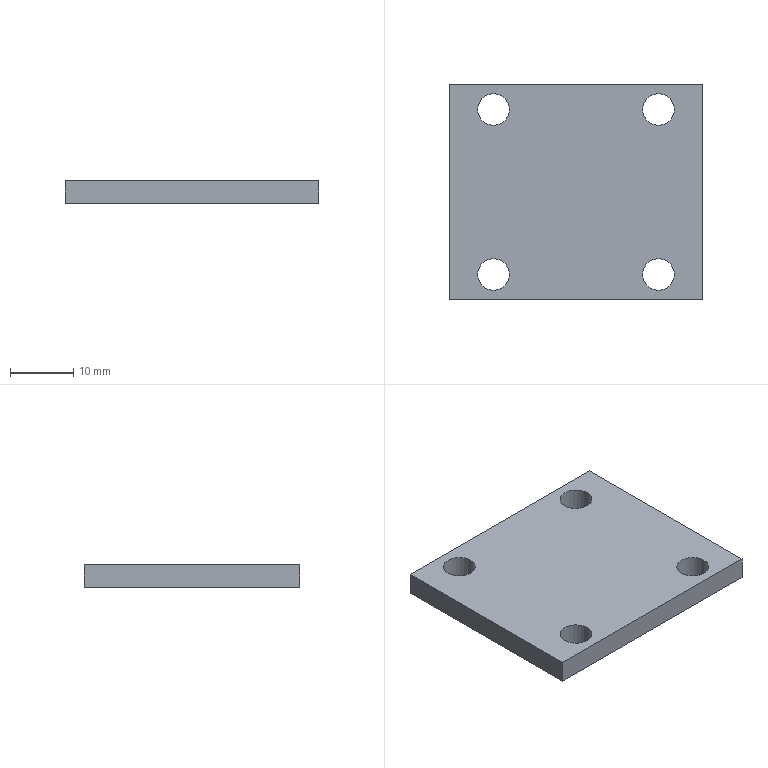Part | NX | 1 solid | 14 faces | box 40 x 34 x 3.6 mm | volume 4613 mm3 | cylinder 8 | plane 6 | commonest cylinder face diameters 5 x8
STEP:
#1=CARTESIAN_POINT('',(0.,0.,-5.));
#2=VERTEX_POINT('',#1);
#3=CARTESIAN_POINT('',(0.,-34.,-5.));
#4=VERTEX_POINT('',#3);
#5=CARTESIAN_POINT('',(0.,0.,-5.));
#6=DIRECTION('',(0.,-1.,0.));
#7=VECTOR('',#6,1000.);
#8=LINE('',#5,#7);
#9=EDGE_CURVE('',#2,#4,#8,.T.);
#10=ORIENTED_EDGE('',*,*,#9,.T.);
#11=CARTESIAN_POINT('',(40.,-34.,-5.));
#12=VERTEX_POINT('',#11);
#13=CARTESIAN_POINT('',(0.,-34.,-5.));
#14=DIRECTION('',(1.,0.,0.));
#15=VECTOR('',#14,1000.);
#16=LINE('',#13,#15);
#17=EDGE_CURVE('',#4,#12,#16,.T.);
#18=ORIENTED_EDGE('',*,*,#17,.T.);
#19=CARTESIAN_POINT('',(40.,0.,-5.));
#20=VERTEX_POINT('',#19);
#21=CARTESIAN_POINT('',(40.,0.,-5.));
#22=DIRECTION('',(0.,1.,0.));
#23=VECTOR('',#22,1000.);
#24=LINE('',#21,#23);
#25=EDGE_CURVE('',#12,#20,#24,.T.);
#26=ORIENTED_EDGE('',*,*,#25,.T.);
#27=CARTESIAN_POINT('',(0.,0.,-5.));
#28=DIRECTION('',(-1.,0.,0.));
#29=VECTOR('',#28,1000.);
#30=LINE('',#27,#29);
#31=EDGE_CURVE('',#20,#2,#30,.T.);
#32=ORIENTED_EDGE('',*,*,#31,.T.);
#33=EDGE_LOOP('',(#10,#18,#26,#32));
#34=FACE_BOUND('',#33,.T.);
#35=CARTESIAN_POINT('',(4.5,-4.,-5.));
#36=VERTEX_POINT('',#35);
#37=CARTESIAN_POINT('',(9.5,-4.,-5.));
#38=VERTEX_POINT('',#37);
#39=CARTESIAN_POINT('',(7.,-4.,-5.));
#40=DIRECTION('',(0.,0.,-1.));
#41=DIRECTION('',(-1.,0.,0.));
#42=AXIS2_PLACEMENT_3D('',#39,#40,#41);
#43=CIRCLE('',#42,2.5);
#44=EDGE_CURVE('',#36,#38,#43,.T.);
#45=ORIENTED_EDGE('',*,*,#44,.T.);
#46=CARTESIAN_POINT('',(7.,-4.,-5.));
#47=DIRECTION('',(0.,0.,-1.));
#48=DIRECTION('',(-1.,0.,0.));
#49=AXIS2_PLACEMENT_3D('',#46,#47,#48);
#50=CIRCLE('',#49,2.5);
#51=EDGE_CURVE('',#38,#36,#50,.T.);
#52=ORIENTED_EDGE('',*,*,#51,.T.);
#53=EDGE_LOOP('',(#45,#52));
#54=FACE_BOUND('',#53,.T.);
#55=CARTESIAN_POINT('',(4.5,-30.,-5.));
#56=VERTEX_POINT('',#55);
#57=CARTESIAN_POINT('',(9.5,-30.,-5.));
#58=VERTEX_POINT('',#57);
#59=CARTESIAN_POINT('',(7.,-30.,-5.));
#60=DIRECTION('',(0.,0.,-1.));
#61=DIRECTION('',(-1.,0.,0.));
#62=AXIS2_PLACEMENT_3D('',#59,#60,#61);
#63=CIRCLE('',#62,2.5);
#64=EDGE_CURVE('',#56,#58,#63,.T.);
#65=ORIENTED_EDGE('',*,*,#64,.T.);
#66=CARTESIAN_POINT('',(7.,-30.,-5.));
#67=DIRECTION('',(0.,0.,-1.));
#68=DIRECTION('',(-1.,0.,0.));
#69=AXIS2_PLACEMENT_3D('',#66,#67,#68);
#70=CIRCLE('',#69,2.5);
#71=EDGE_CURVE('',#58,#56,#70,.T.);
#72=ORIENTED_EDGE('',*,*,#71,.T.);
#73=EDGE_LOOP('',(#65,#72));
#74=FACE_BOUND('',#73,.T.);
#75=CARTESIAN_POINT('',(35.5,-4.,-5.));
#76=VERTEX_POINT('',#75);
#77=CARTESIAN_POINT('',(30.5,-4.,-5.));
#78=VERTEX_POINT('',#77);
#79=CARTESIAN_POINT('',(33.,-4.,-5.));
#80=DIRECTION('',(0.,0.,-1.));
#81=DIRECTION('',(-1.,0.,0.));
#82=AXIS2_PLACEMENT_3D('',#79,#80,#81);
#83=CIRCLE('',#82,2.5);
#84=EDGE_CURVE('',#76,#78,#83,.T.);
#85=ORIENTED_EDGE('',*,*,#84,.T.);
#86=CARTESIAN_POINT('',(33.,-4.,-5.));
#87=DIRECTION('',(0.,0.,-1.));
#88=DIRECTION('',(-1.,0.,0.));
#89=AXIS2_PLACEMENT_3D('',#86,#87,#88);
#90=CIRCLE('',#89,2.5);
#91=EDGE_CURVE('',#78,#76,#90,.T.);
#92=ORIENTED_EDGE('',*,*,#91,.T.);
#93=EDGE_LOOP('',(#85,#92));
#94=FACE_BOUND('',#93,.T.);
#95=CARTESIAN_POINT('',(30.5,-30.,-5.));
#96=VERTEX_POINT('',#95);
#97=CARTESIAN_POINT('',(35.5,-30.,-5.));
#98=VERTEX_POINT('',#97);
#99=CARTESIAN_POINT('',(33.,-30.,-5.));
#100=DIRECTION('',(0.,0.,-1.));
#101=DIRECTION('',(-1.,0.,0.));
#102=AXIS2_PLACEMENT_3D('',#99,#100,#101);
#103=CIRCLE('',#102,2.5);
#104=EDGE_CURVE('',#96,#98,#103,.T.);
#105=ORIENTED_EDGE('',*,*,#104,.T.);
#106=CARTESIAN_POINT('',(33.,-30.,-5.));
#107=DIRECTION('',(0.,0.,-1.));
#108=DIRECTION('',(-1.,0.,0.));
#109=AXIS2_PLACEMENT_3D('',#106,#107,#108);
#110=CIRCLE('',#109,2.5);
#111=EDGE_CURVE('',#98,#96,#110,.T.);
#112=ORIENTED_EDGE('',*,*,#111,.T.);
#113=EDGE_LOOP('',(#105,#112));
#114=FACE_BOUND('',#113,.T.);
#115=CARTESIAN_POINT('',(0.,0.,-5.));
#116=DIRECTION('',(0.,0.,1.));
#117=DIRECTION('',(1.,0.,0.));
#118=AXIS2_PLACEMENT_3D('',#115,#116,#117);
#119=PLANE('',#118);
#120=ADVANCED_FACE('',(#34,#54,#74,#94,#114),#119,.T.);
#121=CARTESIAN_POINT('',(0.,0.,-8.6));
#122=VERTEX_POINT('',#121);
#123=CARTESIAN_POINT('',(0.,-34.,-8.6));
#124=VERTEX_POINT('',#123);
#125=CARTESIAN_POINT('',(0.,0.,-8.6));
#126=DIRECTION('',(0.,-1.,0.));
#127=VECTOR('',#126,1000.);
#128=LINE('',#125,#127);
#129=EDGE_CURVE('',#122,#124,#128,.T.);
#130=ORIENTED_EDGE('',*,*,#129,.T.);
#131=CARTESIAN_POINT('',(0.,-34.,0.));
#132=DIRECTION('',(0.,0.,-1.));
#133=VECTOR('',#132,1000.);
#134=LINE('',#131,#133);
#135=EDGE_CURVE('',#4,#124,#134,.T.);
#136=ORIENTED_EDGE('',*,*,#135,.F.);
#137=ORIENTED_EDGE('',*,*,#9,.F.);
#138=CARTESIAN_POINT('',(0.,0.,0.));
#139=DIRECTION('',(0.,0.,1.));
#140=VECTOR('',#139,1000.);
#141=LINE('',#138,#140);
#142=EDGE_CURVE('',#122,#2,#141,.T.);
#143=ORIENTED_EDGE('',*,*,#142,.F.);
#144=EDGE_LOOP('',(#130,#136,#137,#143));
#145=FACE_BOUND('',#144,.T.);
#146=CARTESIAN_POINT('',(0.,0.,0.));
#147=DIRECTION('',(-1.,0.,0.));
#148=DIRECTION('',(0.,0.,1.));
#149=AXIS2_PLACEMENT_3D('',#146,#147,#148);
#150=PLANE('',#149);
#151=ADVANCED_FACE('',(#145),#150,.T.);
#152=CARTESIAN_POINT('',(40.,0.,-8.6));
#153=VERTEX_POINT('',#152);
#154=CARTESIAN_POINT('',(0.,0.,-8.6));
#155=DIRECTION('',(-1.,0.,0.));
#156=VECTOR('',#155,1000.);
#157=LINE('',#154,#156);
#158=EDGE_CURVE('',#153,#122,#157,.T.);
#159=ORIENTED_EDGE('',*,*,#158,.T.);
#160=ORIENTED_EDGE('',*,*,#142,.T.);
#161=ORIENTED_EDGE('',*,*,#31,.F.);
#162=CARTESIAN_POINT('',(40.,0.,0.));
#163=DIRECTION('',(0.,0.,-1.));
#164=VECTOR('',#163,1000.);
#165=LINE('',#162,#164);
#166=EDGE_CURVE('',#20,#153,#165,.T.);
#167=ORIENTED_EDGE('',*,*,#166,.T.);
#168=EDGE_LOOP('',(#159,#160,#161,#167));
#169=FACE_BOUND('',#168,.T.);
#170=CARTESIAN_POINT('',(40.,0.,0.));
#171=DIRECTION('',(0.,1.,0.));
#172=DIRECTION('',(1.,0.,0.));
#173=AXIS2_PLACEMENT_3D('',#170,#171,#172);
#174=PLANE('',#173);
#175=ADVANCED_FACE('',(#169),#174,.T.);
#176=CARTESIAN_POINT('',(40.,-34.,-8.6));
#177=VERTEX_POINT('',#176);
#178=CARTESIAN_POINT('',(40.,0.,-8.6));
#179=DIRECTION('',(0.,1.,0.));
#180=VECTOR('',#179,1000.);
#181=LINE('',#178,#180);
#182=EDGE_CURVE('',#177,#153,#181,.T.);
#183=ORIENTED_EDGE('',*,*,#182,.T.);
#184=ORIENTED_EDGE('',*,*,#166,.F.);
#185=ORIENTED_EDGE('',*,*,#25,.F.);
#186=CARTESIAN_POINT('',(40.,-34.,0.));
#187=DIRECTION('',(0.,0.,1.));
#188=VECTOR('',#187,1000.);
#189=LINE('',#186,#188);
#190=EDGE_CURVE('',#177,#12,#189,.T.);
#191=ORIENTED_EDGE('',*,*,#190,.F.);
#192=EDGE_LOOP('',(#183,#184,#185,#191));
#193=FACE_BOUND('',#192,.T.);
#194=CARTESIAN_POINT('',(40.,-34.,0.));
#195=DIRECTION('',(1.,0.,0.));
#196=DIRECTION('',(0.,1.,0.));
#197=AXIS2_PLACEMENT_3D('',#194,#195,#196);
#198=PLANE('',#197);
#199=ADVANCED_FACE('',(#193),#198,.T.);
#200=CARTESIAN_POINT('',(0.,-34.,-8.6));
#201=DIRECTION('',(1.,0.,0.));
#202=VECTOR('',#201,1000.);
#203=LINE('',#200,#202);
#204=EDGE_CURVE('',#124,#177,#203,.T.);
#205=ORIENTED_EDGE('',*,*,#204,.T.);
#206=ORIENTED_EDGE('',*,*,#190,.T.);
#207=ORIENTED_EDGE('',*,*,#17,.F.);
#208=ORIENTED_EDGE('',*,*,#135,.T.);
#209=EDGE_LOOP('',(#205,#206,#207,#208));
#210=FACE_BOUND('',#209,.T.);
#211=CARTESIAN_POINT('',(0.,-34.,0.));
#212=DIRECTION('',(0.,-1.,0.));
#213=DIRECTION('',(0.,0.,-1.));
#214=AXIS2_PLACEMENT_3D('',#211,#212,#213);
#215=PLANE('',#214);
#216=ADVANCED_FACE('',(#210),#215,.T.);
#217=ORIENTED_EDGE('',*,*,#129,.F.);
#218=ORIENTED_EDGE('',*,*,#158,.F.);
#219=ORIENTED_EDGE('',*,*,#182,.F.);
#220=ORIENTED_EDGE('',*,*,#204,.F.);
#221=EDGE_LOOP('',(#217,#218,#219,#220));
#222=FACE_BOUND('',#221,.T.);
#223=CARTESIAN_POINT('',(9.5,-4.,-8.6));
#224=VERTEX_POINT('',#223);
#225=CARTESIAN_POINT('',(4.5,-4.,-8.6));
#226=VERTEX_POINT('',#225);
#227=CARTESIAN_POINT('',(7.,-4.,-8.6));
#228=DIRECTION('',(0.,0.,-1.));
#229=DIRECTION('',(-1.,0.,0.));
#230=AXIS2_PLACEMENT_3D('',#227,#228,#229);
#231=CIRCLE('',#230,2.5);
#232=EDGE_CURVE('',#224,#226,#231,.T.);
#233=ORIENTED_EDGE('',*,*,#232,.F.);
#234=CARTESIAN_POINT('',(7.,-4.,-8.6));
#235=DIRECTION('',(0.,0.,-1.));
#236=DIRECTION('',(-1.,0.,0.));
#237=AXIS2_PLACEMENT_3D('',#234,#235,#236);
#238=CIRCLE('',#237,2.5);
#239=EDGE_CURVE('',#226,#224,#238,.T.);
#240=ORIENTED_EDGE('',*,*,#239,.F.);
#241=EDGE_LOOP('',(#233,#240));
#242=FACE_BOUND('',#241,.T.);
#243=CARTESIAN_POINT('',(4.5,-30.,-8.6));
#244=VERTEX_POINT('',#243);
#245=CARTESIAN_POINT('',(9.5,-30.,-8.6));
#246=VERTEX_POINT('',#245);
#247=CARTESIAN_POINT('',(7.,-30.,-8.6));
#248=DIRECTION('',(0.,0.,-1.));
#249=DIRECTION('',(-1.,0.,0.));
#250=AXIS2_PLACEMENT_3D('',#247,#248,#249);
#251=CIRCLE('',#250,2.5);
#252=EDGE_CURVE('',#244,#246,#251,.T.);
#253=ORIENTED_EDGE('',*,*,#252,.F.);
#254=CARTESIAN_POINT('',(7.,-30.,-8.6));
#255=DIRECTION('',(0.,0.,-1.));
#256=DIRECTION('',(-1.,0.,0.));
#257=AXIS2_PLACEMENT_3D('',#254,#255,#256);
#258=CIRCLE('',#257,2.5);
#259=EDGE_CURVE('',#246,#244,#258,.T.);
#260=ORIENTED_EDGE('',*,*,#259,.F.);
#261=EDGE_LOOP('',(#253,#260));
#262=FACE_BOUND('',#261,.T.);
#263=CARTESIAN_POINT('',(35.5,-4.,-8.6));
#264=VERTEX_POINT('',#263);
#265=CARTESIAN_POINT('',(30.5,-4.,-8.6));
#266=VERTEX_POINT('',#265);
#267=CARTESIAN_POINT('',(33.,-4.,-8.6));
#268=DIRECTION('',(0.,0.,-1.));
#269=DIRECTION('',(-1.,0.,0.));
#270=AXIS2_PLACEMENT_3D('',#267,#268,#269);
#271=CIRCLE('',#270,2.5);
#272=EDGE_CURVE('',#264,#266,#271,.T.);
#273=ORIENTED_EDGE('',*,*,#272,.F.);
#274=CARTESIAN_POINT('',(33.,-4.,-8.6));
#275=DIRECTION('',(0.,0.,-1.));
#276=DIRECTION('',(-1.,0.,0.));
#277=AXIS2_PLACEMENT_3D('',#274,#275,#276);
#278=CIRCLE('',#277,2.5);
#279=EDGE_CURVE('',#266,#264,#278,.T.);
#280=ORIENTED_EDGE('',*,*,#279,.F.);
#281=EDGE_LOOP('',(#273,#280));
#282=FACE_BOUND('',#281,.T.);
#283=CARTESIAN_POINT('',(35.5,-30.,-8.6));
#284=VERTEX_POINT('',#283);
#285=CARTESIAN_POINT('',(30.5,-30.,-8.6));
#286=VERTEX_POINT('',#285);
#287=CARTESIAN_POINT('',(33.,-30.,-8.6));
#288=DIRECTION('',(0.,0.,-1.));
#289=DIRECTION('',(-1.,0.,0.));
#290=AXIS2_PLACEMENT_3D('',#287,#288,#289);
#291=CIRCLE('',#290,2.5);
#292=EDGE_CURVE('',#284,#286,#291,.T.);
#293=ORIENTED_EDGE('',*,*,#292,.F.);
#294=CARTESIAN_POINT('',(33.,-30.,-8.6));
#295=DIRECTION('',(0.,0.,-1.));
#296=DIRECTION('',(-1.,0.,0.));
#297=AXIS2_PLACEMENT_3D('',#294,#295,#296);
#298=CIRCLE('',#297,2.5);
#299=EDGE_CURVE('',#286,#284,#298,.T.);
#300=ORIENTED_EDGE('',*,*,#299,.F.);
#301=EDGE_LOOP('',(#293,#300));
#302=FACE_BOUND('',#301,.T.);
#303=CARTESIAN_POINT('',(0.,0.,-8.6));
#304=DIRECTION('',(0.,0.,1.));
#305=DIRECTION('',(1.,0.,0.));
#306=AXIS2_PLACEMENT_3D('',#303,#304,#305);
#307=PLANE('',#306);
#308=ADVANCED_FACE('',(#222,#242,#262,#282,#302),#307,.F.);
#309=ORIENTED_EDGE('',*,*,#232,.T.);
#310=CARTESIAN_POINT('',(4.5,-4.,3.7));
#311=DIRECTION('',(0.,0.,-1.));
#312=VECTOR('',#311,1000.);
#313=LINE('',#310,#312);
#314=EDGE_CURVE('',#226,#36,#313,.F.);
#315=ORIENTED_EDGE('',*,*,#314,.T.);
#316=ORIENTED_EDGE('',*,*,#51,.F.);
#317=CARTESIAN_POINT('',(9.5,-4.,3.7));
#318=DIRECTION('',(0.,0.,-1.));
#319=VECTOR('',#318,1000.);
#320=LINE('',#317,#319);
#321=EDGE_CURVE('',#224,#38,#320,.F.);
#322=ORIENTED_EDGE('',*,*,#321,.F.);
#323=EDGE_LOOP('',(#309,#315,#316,#322));
#324=FACE_BOUND('',#323,.T.);
#325=CARTESIAN_POINT('',(7.,-4.,3.7));
#326=DIRECTION('',(0.,0.,-1.));
#327=DIRECTION('',(-1.,0.,0.));
#328=AXIS2_PLACEMENT_3D('',#325,#326,#327);
#329=CYLINDRICAL_SURFACE('',#328,2.5);
#330=ADVANCED_FACE('',(#324),#329,.F.);
#331=ORIENTED_EDGE('',*,*,#272,.T.);
#332=CARTESIAN_POINT('',(30.5,-4.,3.7));
#333=DIRECTION('',(0.,0.,-1.));
#334=VECTOR('',#333,1000.);
#335=LINE('',#332,#334);
#336=EDGE_CURVE('',#266,#78,#335,.F.);
#337=ORIENTED_EDGE('',*,*,#336,.T.);
#338=ORIENTED_EDGE('',*,*,#84,.F.);
#339=CARTESIAN_POINT('',(35.5,-4.,3.7));
#340=DIRECTION('',(0.,0.,-1.));
#341=VECTOR('',#340,1000.);
#342=LINE('',#339,#341);
#343=EDGE_CURVE('',#264,#76,#342,.F.);
#344=ORIENTED_EDGE('',*,*,#343,.F.);
#345=EDGE_LOOP('',(#331,#337,#338,#344));
#346=FACE_BOUND('',#345,.T.);
#347=CARTESIAN_POINT('',(33.,-4.,3.7));
#348=DIRECTION('',(0.,0.,-1.));
#349=DIRECTION('',(-1.,0.,0.));
#350=AXIS2_PLACEMENT_3D('',#347,#348,#349);
#351=CYLINDRICAL_SURFACE('',#350,2.5);
#352=ADVANCED_FACE('',(#346),#351,.F.);
#353=ORIENTED_EDGE('',*,*,#64,.F.);
#354=CARTESIAN_POINT('',(4.5,-30.,3.7));
#355=DIRECTION('',(0.,0.,-1.));
#356=VECTOR('',#355,1000.);
#357=LINE('',#354,#356);
#358=EDGE_CURVE('',#244,#56,#357,.F.);
#359=ORIENTED_EDGE('',*,*,#358,.F.);
#360=ORIENTED_EDGE('',*,*,#252,.T.);
#361=CARTESIAN_POINT('',(9.5,-30.,3.7));
#362=DIRECTION('',(0.,0.,-1.));
#363=VECTOR('',#362,1000.);
#364=LINE('',#361,#363);
#365=EDGE_CURVE('',#246,#58,#364,.F.);
#366=ORIENTED_EDGE('',*,*,#365,.T.);
#367=EDGE_LOOP('',(#353,#359,#360,#366));
#368=FACE_BOUND('',#367,.T.);
#369=CARTESIAN_POINT('',(7.,-30.,3.7));
#370=DIRECTION('',(0.,0.,-1.));
#371=DIRECTION('',(-1.,0.,0.));
#372=AXIS2_PLACEMENT_3D('',#369,#370,#371);
#373=CYLINDRICAL_SURFACE('',#372,2.5);
#374=ADVANCED_FACE('',(#368),#373,.F.);
#375=ORIENTED_EDGE('',*,*,#104,.F.);
#376=CARTESIAN_POINT('',(30.5,-30.,3.7));
#377=DIRECTION('',(0.,0.,-1.));
#378=VECTOR('',#377,1000.);
#379=LINE('',#376,#378);
#380=EDGE_CURVE('',#286,#96,#379,.F.);
#381=ORIENTED_EDGE('',*,*,#380,.F.);
#382=ORIENTED_EDGE('',*,*,#299,.T.);
#383=CARTESIAN_POINT('',(35.5,-30.,3.7));
#384=DIRECTION('',(0.,0.,-1.));
#385=VECTOR('',#384,1000.);
#386=LINE('',#383,#385);
#387=EDGE_CURVE('',#284,#98,#386,.F.);
#388=ORIENTED_EDGE('',*,*,#387,.T.);
#389=EDGE_LOOP('',(#375,#381,#382,#388));
#390=FACE_BOUND('',#389,.T.);
#391=CARTESIAN_POINT('',(33.,-30.,3.7));
#392=DIRECTION('',(0.,0.,-1.));
#393=DIRECTION('',(-1.,0.,0.));
#394=AXIS2_PLACEMENT_3D('',#391,#392,#393);
#395=CYLINDRICAL_SURFACE('',#394,2.5);
#396=ADVANCED_FACE('',(#390),#395,.F.);
#397=ORIENTED_EDGE('',*,*,#292,.T.);
#398=ORIENTED_EDGE('',*,*,#380,.T.);
#399=ORIENTED_EDGE('',*,*,#111,.F.);
#400=ORIENTED_EDGE('',*,*,#387,.F.);
#401=EDGE_LOOP('',(#397,#398,#399,#400));
#402=FACE_BOUND('',#401,.T.);
#403=CARTESIAN_POINT('',(33.,-30.,3.7));
#404=DIRECTION('',(0.,0.,-1.));
#405=DIRECTION('',(-1.,0.,0.));
#406=AXIS2_PLACEMENT_3D('',#403,#404,#405);
#407=CYLINDRICAL_SURFACE('',#406,2.5);
#408=ADVANCED_FACE('',(#402),#407,.F.);
#409=ORIENTED_EDGE('',*,*,#336,.F.);
#410=ORIENTED_EDGE('',*,*,#279,.T.);
#411=ORIENTED_EDGE('',*,*,#343,.T.);
#412=ORIENTED_EDGE('',*,*,#91,.F.);
#413=EDGE_LOOP('',(#409,#410,#411,#412));
#414=FACE_BOUND('',#413,.T.);
#415=CARTESIAN_POINT('',(33.,-4.,3.7));
#416=DIRECTION('',(0.,0.,-1.));
#417=DIRECTION('',(-1.,0.,0.));
#418=AXIS2_PLACEMENT_3D('',#415,#416,#417);
#419=CYLINDRICAL_SURFACE('',#418,2.5);
#420=ADVANCED_FACE('',(#414),#419,.F.);
#421=ORIENTED_EDGE('',*,*,#358,.T.);
#422=ORIENTED_EDGE('',*,*,#71,.F.);
#423=ORIENTED_EDGE('',*,*,#365,.F.);
#424=ORIENTED_EDGE('',*,*,#259,.T.);
#425=EDGE_LOOP('',(#421,#422,#423,#424));
#426=FACE_BOUND('',#425,.T.);
#427=CARTESIAN_POINT('',(7.,-30.,3.7));
#428=DIRECTION('',(0.,0.,-1.));
#429=DIRECTION('',(-1.,0.,0.));
#430=AXIS2_PLACEMENT_3D('',#427,#428,#429);
#431=CYLINDRICAL_SURFACE('',#430,2.5);
#432=ADVANCED_FACE('',(#426),#431,.F.);
#433=ORIENTED_EDGE('',*,*,#44,.F.);
#434=ORIENTED_EDGE('',*,*,#314,.F.);
#435=ORIENTED_EDGE('',*,*,#239,.T.);
#436=ORIENTED_EDGE('',*,*,#321,.T.);
#437=EDGE_LOOP('',(#433,#434,#435,#436));
#438=FACE_BOUND('',#437,.T.);
#439=CARTESIAN_POINT('',(7.,-4.,3.7));
#440=DIRECTION('',(0.,0.,-1.));
#441=DIRECTION('',(-1.,0.,0.));
#442=AXIS2_PLACEMENT_3D('',#439,#440,#441);
#443=CYLINDRICAL_SURFACE('',#442,2.5);
#444=ADVANCED_FACE('',(#438),#443,.F.);
#445=CLOSED_SHELL('',(#120,#151,#175,#199,#216,#308,#330,#352,#374,#396,#408,#420,#432,#444));
#446=MANIFOLD_SOLID_BREP('',#445);
#447=(LENGTH_UNIT()NAMED_UNIT(*)SI_UNIT(.MILLI.,.METRE.));
#448=UNCERTAINTY_MEASURE_WITH_UNIT(LENGTH_MEASURE(0.00001),#447,'','');
#449=(NAMED_UNIT(*)PLANE_ANGLE_UNIT()SI_UNIT($,.RADIAN.));
#450=(NAMED_UNIT(*)SI_UNIT($,.STERADIAN.)SOLID_ANGLE_UNIT());
#451=(GEOMETRIC_REPRESENTATION_CONTEXT(3)GLOBAL_UNCERTAINTY_ASSIGNED_CONTEXT((#448))GLOBAL_UNIT_ASSIGNED_CONTEXT((#447,#449,#450))REPRESENTATION_CONTEXT('',''));
#452=ADVANCED_BREP_SHAPE_REPRESENTATION('',(#446),#451);